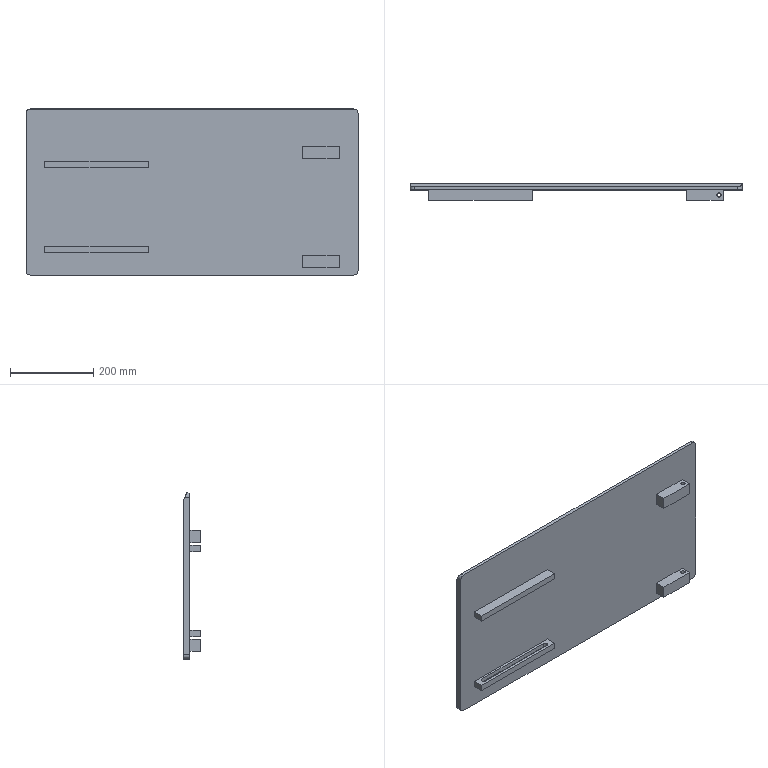Part | SolidWorks | features ICE 4, Cut 2, Fillet 2, MirrorPattern 2, Draft 1, Extrusion 1 | 1 solid | 60 faces | box 800 x 40 x 400.131 mm | volume 4882709 mm3 | plane 36 | cylinder 20 | torus 4 | commonest cylinder face diameters 12 x6 4 x4 10 x4 20 x4 40 x2